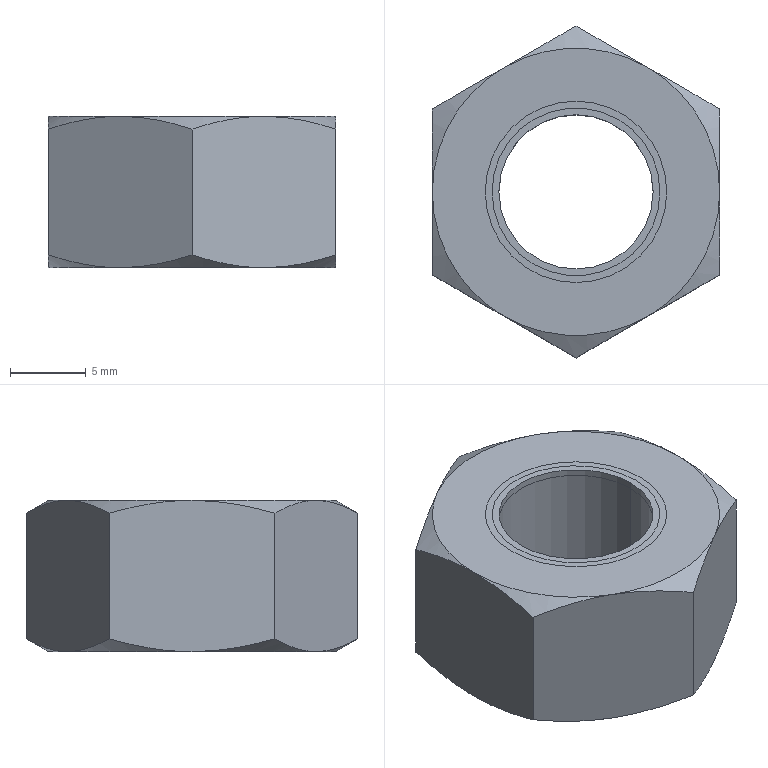Part | STEP file | M12 | 2 solids | 32 faces | box 19 x 21.939 x 10 mm | volume 2601 mm3 | cone 16 | plane 10 | cylinder 6 | commonest cylinder face diameters 10.2 x4 12 x2
STEP:
#1=CARTESIAN_POINT('',(5.1,0.,9.55));
#2=VERTEX_POINT('',#1);
#3=CARTESIAN_POINT('',(-5.1,0.,9.55));
#4=VERTEX_POINT('',#3);
#5=CARTESIAN_POINT('',(0.,0.,9.55));
#6=DIRECTION('',(0.,0.,-1.));
#7=DIRECTION('',(1.,0.,0.));
#8=AXIS2_PLACEMENT_3D('',#5,#6,#7);
#9=CIRCLE('',#8,5.1);
#10=EDGE_CURVE('',#2,#4,#9,.T.);
#11=ORIENTED_EDGE('',*,*,#10,.F.);
#12=CARTESIAN_POINT('',(5.1,0.,0.45));
#13=VERTEX_POINT('',#12);
#14=CARTESIAN_POINT('',(5.1,0.,0.));
#15=DIRECTION('',(0.,0.,-1.));
#16=VECTOR('',#15,1000.);
#17=LINE('',#14,#16);
#18=EDGE_CURVE('',#2,#13,#17,.T.);
#19=ORIENTED_EDGE('',*,*,#18,.T.);
#20=CARTESIAN_POINT('',(-5.1,0.,0.45));
#21=VERTEX_POINT('',#20);
#22=CARTESIAN_POINT('',(0.,0.,0.45));
#23=DIRECTION('',(0.,0.,1.));
#24=DIRECTION('',(-1.,0.,0.));
#25=AXIS2_PLACEMENT_3D('',#22,#23,#24);
#26=CIRCLE('',#25,5.1);
#27=EDGE_CURVE('',#21,#13,#26,.T.);
#28=ORIENTED_EDGE('',*,*,#27,.F.);
#29=CARTESIAN_POINT('',(-5.1,0.,0.));
#30=DIRECTION('',(0.,0.,-1.));
#31=VECTOR('',#30,1000.);
#32=LINE('',#29,#31);
#33=EDGE_CURVE('',#4,#21,#32,.T.);
#34=ORIENTED_EDGE('',*,*,#33,.F.);
#35=EDGE_LOOP('',(#11,#19,#28,#34));
#36=FACE_OUTER_BOUND('',#35,.T.);
#37=CARTESIAN_POINT('',(0.,0.,0.));
#38=DIRECTION('',(0.,0.,-1.));
#39=DIRECTION('',(-1.,0.,0.));
#40=AXIS2_PLACEMENT_3D('',#37,#38,#39);
#41=CYLINDRICAL_SURFACE('',#40,5.1);
#42=ADVANCED_FACE('',(#36),#41,.F.);
#43=ORIENTED_EDGE('',*,*,#27,.T.);
#44=CARTESIAN_POINT('',(5.55,0.,0.));
#45=VERTEX_POINT('',#44);
#46=CARTESIAN_POINT('',(5.55,0.,0.000002816));
#47=DIRECTION('',(0.7071,0.,-0.7071));
#48=VECTOR('',#47,1000.);
#49=LINE('',#46,#48);
#50=EDGE_CURVE('',#13,#45,#49,.T.);
#51=ORIENTED_EDGE('',*,*,#50,.T.);
#52=CARTESIAN_POINT('',(-5.55,0.,0.));
#53=VERTEX_POINT('',#52);
#54=CARTESIAN_POINT('',(0.,0.,0.));
#55=DIRECTION('',(0.,0.,-1.));
#56=DIRECTION('',(1.,0.,0.));
#57=AXIS2_PLACEMENT_3D('',#54,#55,#56);
#58=CIRCLE('',#57,5.55);
#59=EDGE_CURVE('',#45,#53,#58,.T.);
#60=ORIENTED_EDGE('',*,*,#59,.T.);
#61=CARTESIAN_POINT('',(-5.55,0.,0.000002816));
#62=DIRECTION('',(-0.7071,0.,-0.7071));
#63=VECTOR('',#62,1000.);
#64=LINE('',#61,#63);
#65=EDGE_CURVE('',#21,#53,#64,.T.);
#66=ORIENTED_EDGE('',*,*,#65,.F.);
#67=EDGE_LOOP('',(#43,#51,#60,#66));
#68=FACE_OUTER_BOUND('',#67,.T.);
#69=CARTESIAN_POINT('',(0.,0.,0.000002816));
#70=DIRECTION('',(0.,0.,-1.));
#71=DIRECTION('',(-1.,0.,0.));
#72=AXIS2_PLACEMENT_3D('',#69,#70,#71);
#73=CONICAL_SURFACE('',#72,5.55,0.7854);
#74=ADVANCED_FACE('',(#68),#73,.F.);
#75=ORIENTED_EDGE('',*,*,#10,.T.);
#76=CARTESIAN_POINT('',(-5.55,0.,10.));
#77=VERTEX_POINT('',#76);
#78=CARTESIAN_POINT('',(-5.55,0.,10.));
#79=DIRECTION('',(-0.7071,0.,0.7071));
#80=VECTOR('',#79,1000.);
#81=LINE('',#78,#80);
#82=EDGE_CURVE('',#4,#77,#81,.T.);
#83=ORIENTED_EDGE('',*,*,#82,.T.);
#84=CARTESIAN_POINT('',(5.55,0.,10.));
#85=VERTEX_POINT('',#84);
#86=CARTESIAN_POINT('',(0.,0.,10.));
#87=DIRECTION('',(0.,0.,-1.));
#88=DIRECTION('',(1.,0.,0.));
#89=AXIS2_PLACEMENT_3D('',#86,#87,#88);
#90=CIRCLE('',#89,5.55);
#91=EDGE_CURVE('',#85,#77,#90,.T.);
#92=ORIENTED_EDGE('',*,*,#91,.F.);
#93=CARTESIAN_POINT('',(5.55,0.,10.));
#94=DIRECTION('',(0.7071,0.,0.7071));
#95=VECTOR('',#94,1000.);
#96=LINE('',#93,#95);
#97=EDGE_CURVE('',#2,#85,#96,.T.);
#98=ORIENTED_EDGE('',*,*,#97,.F.);
#99=EDGE_LOOP('',(#75,#83,#92,#98));
#100=FACE_OUTER_BOUND('',#99,.T.);
#101=CARTESIAN_POINT('',(0.,0.,10.));
#102=DIRECTION('',(0.,0.,1.));
#103=DIRECTION('',(1.,0.,0.));
#104=AXIS2_PLACEMENT_3D('',#101,#102,#103);
#105=CONICAL_SURFACE('',#104,5.55,0.7854);
#106=ADVANCED_FACE('',(#100),#105,.F.);
#107=CARTESIAN_POINT('',(0.,0.,0.));
#108=DIRECTION('',(0.,0.,-1.));
#109=DIRECTION('',(1.,0.,0.));
#110=AXIS2_PLACEMENT_3D('',#107,#108,#109);
#111=CIRCLE('',#110,5.55);
#112=EDGE_CURVE('',#53,#45,#111,.T.);
#113=ORIENTED_EDGE('',*,*,#112,.F.);
#114=ORIENTED_EDGE('',*,*,#59,.F.);
#115=EDGE_LOOP('',(#113,#114));
#116=FACE_BOUND('',#115,.T.);
#117=CARTESIAN_POINT('',(-4.75,8.227,0.));
#118=VERTEX_POINT('',#117);
#119=CARTESIAN_POINT('',(-9.5,0.,0.));
#120=VERTEX_POINT('',#119);
#121=CARTESIAN_POINT('',(0.,0.,0.));
#122=DIRECTION('',(0.,0.,1.));
#123=DIRECTION('',(1.,0.,0.));
#124=AXIS2_PLACEMENT_3D('',#121,#122,#123);
#125=CIRCLE('',#124,9.5);
#126=EDGE_CURVE('',#118,#120,#125,.T.);
#127=ORIENTED_EDGE('',*,*,#126,.F.);
#128=CARTESIAN_POINT('',(4.75,8.227,0.));
#129=VERTEX_POINT('',#128);
#130=CARTESIAN_POINT('',(0.,0.,0.));
#131=DIRECTION('',(0.,0.,1.));
#132=DIRECTION('',(1.,0.,0.));
#133=AXIS2_PLACEMENT_3D('',#130,#131,#132);
#134=CIRCLE('',#133,9.5);
#135=EDGE_CURVE('',#129,#118,#134,.T.);
#136=ORIENTED_EDGE('',*,*,#135,.F.);
#137=CARTESIAN_POINT('',(9.5,0.000000041,0.));
#138=VERTEX_POINT('',#137);
#139=CARTESIAN_POINT('',(0.,0.,0.000000001));
#140=DIRECTION('',(0.,0.,1.));
#141=DIRECTION('',(1.,0.,0.));
#142=AXIS2_PLACEMENT_3D('',#139,#140,#141);
#143=CIRCLE('',#142,9.5);
#144=EDGE_CURVE('',#138,#129,#143,.T.);
#145=ORIENTED_EDGE('',*,*,#144,.F.);
#146=CARTESIAN_POINT('',(4.75,-8.227,0.));
#147=VERTEX_POINT('',#146);
#148=CARTESIAN_POINT('',(0.,0.,0.));
#149=DIRECTION('',(0.,0.,1.));
#150=DIRECTION('',(1.,0.,0.));
#151=AXIS2_PLACEMENT_3D('',#148,#149,#150);
#152=CIRCLE('',#151,9.5);
#153=EDGE_CURVE('',#147,#138,#152,.T.);
#154=ORIENTED_EDGE('',*,*,#153,.F.);
#155=CARTESIAN_POINT('',(-4.75,-8.227,0.));
#156=VERTEX_POINT('',#155);
#157=CARTESIAN_POINT('',(0.,0.,0.));
#158=DIRECTION('',(0.,0.,1.));
#159=DIRECTION('',(1.,0.,0.));
#160=AXIS2_PLACEMENT_3D('',#157,#158,#159);
#161=CIRCLE('',#160,9.5);
#162=EDGE_CURVE('',#156,#147,#161,.T.);
#163=ORIENTED_EDGE('',*,*,#162,.F.);
#164=CARTESIAN_POINT('',(0.,0.,0.));
#165=DIRECTION('',(0.,0.,1.));
#166=DIRECTION('',(1.,0.,0.));
#167=AXIS2_PLACEMENT_3D('',#164,#165,#166);
#168=CIRCLE('',#167,9.5);
#169=EDGE_CURVE('',#120,#156,#168,.T.);
#170=ORIENTED_EDGE('',*,*,#169,.F.);
#171=EDGE_LOOP('',(#127,#136,#145,#154,#163,#170));
#172=FACE_OUTER_BOUND('',#171,.T.);
#173=CARTESIAN_POINT('',(0.,0.,0.));
#174=DIRECTION('',(0.,0.,1.));
#175=DIRECTION('',(1.,0.,0.));
#176=AXIS2_PLACEMENT_3D('',#173,#174,#175);
#177=PLANE('',#176);
#178=ADVANCED_FACE('',(#116,#172),#177,.F.);
#179=ORIENTED_EDGE('',*,*,#50,.F.);
#180=CARTESIAN_POINT('',(0.,0.,0.45));
#181=DIRECTION('',(0.,0.,1.));
#182=DIRECTION('',(-1.,0.,0.));
#183=AXIS2_PLACEMENT_3D('',#180,#181,#182);
#184=CIRCLE('',#183,5.1);
#185=EDGE_CURVE('',#13,#21,#184,.T.);
#186=ORIENTED_EDGE('',*,*,#185,.T.);
#187=ORIENTED_EDGE('',*,*,#65,.T.);
#188=ORIENTED_EDGE('',*,*,#112,.T.);
#189=EDGE_LOOP('',(#179,#186,#187,#188));
#190=FACE_OUTER_BOUND('',#189,.T.);
#191=CARTESIAN_POINT('',(0.,0.,0.000002816));
#192=DIRECTION('',(0.,0.,-1.));
#193=DIRECTION('',(-1.,0.,0.));
#194=AXIS2_PLACEMENT_3D('',#191,#192,#193);
#195=CONICAL_SURFACE('',#194,5.55,0.7854);
#196=ADVANCED_FACE('',(#190),#195,.F.);
#197=CARTESIAN_POINT('',(-9.5,-5.485,0.8485));
#198=VERTEX_POINT('',#197);
#199=CARTESIAN_POINT('',(-4.75,-8.227,0.));
#200=CARTESIAN_POINT('',(-5.561,-7.759,0.));
#201=CARTESIAN_POINT('',(-6.36,-7.298,0.08112));
#202=CARTESIAN_POINT('',(-7.942,-6.384,0.3765));
#203=CARTESIAN_POINT('',(-8.724,-5.933,0.5899));
#204=CARTESIAN_POINT('',(-9.5,-5.485,0.8485));
#205=B_SPLINE_CURVE_WITH_KNOTS('',3,(#199,#200,#201,#202,#203,#204),.UNSPECIFIED.,.F.,.F.,(4,2,4),(0.,0.002775,0.00555),.UNSPECIFIED.);
#206=EDGE_CURVE('',#156,#198,#205,.T.);
#207=ORIENTED_EDGE('',*,*,#206,.T.);
#208=CARTESIAN_POINT('',(-9.5,-5.485,0.8485));
#209=CARTESIAN_POINT('',(-9.5,-4.589,0.5899));
#210=CARTESIAN_POINT('',(-9.5,-3.686,0.3765));
#211=CARTESIAN_POINT('',(-9.5,-1.859,0.08112));
#212=CARTESIAN_POINT('',(-9.5,-0.936,0.));
#213=CARTESIAN_POINT('',(-9.5,0.,0.));
#214=B_SPLINE_CURVE_WITH_KNOTS('',3,(#208,#209,#210,#211,#212,#213),.UNSPECIFIED.,.F.,.F.,(4,2,4),(0.,0.002775,0.00555),.UNSPECIFIED.);
#215=EDGE_CURVE('',#198,#120,#214,.T.);
#216=ORIENTED_EDGE('',*,*,#215,.T.);
#217=ORIENTED_EDGE('',*,*,#169,.T.);
#218=EDGE_LOOP('',(#207,#216,#217));
#219=FACE_OUTER_BOUND('',#218,.T.);
#220=CARTESIAN_POINT('',(0.,0.,0.8536));
#221=DIRECTION('',(0.,0.,1.));
#222=DIRECTION('',(1.,0.,0.));
#223=AXIS2_PLACEMENT_3D('',#220,#221,#222);
#224=CONICAL_SURFACE('',#223,10.978,1.047);
#225=ADVANCED_FACE('',(#219),#224,.T.);
#226=CARTESIAN_POINT('',(-9.5,5.485,0.8485));
#227=VERTEX_POINT('',#226);
#228=CARTESIAN_POINT('',(-9.5,0.,0.));
#229=CARTESIAN_POINT('',(-9.5,0.936,0.));
#230=CARTESIAN_POINT('',(-9.5,1.859,0.08112));
#231=CARTESIAN_POINT('',(-9.5,3.686,0.3765));
#232=CARTESIAN_POINT('',(-9.5,4.589,0.5899));
#233=CARTESIAN_POINT('',(-9.5,5.485,0.8485));
#234=B_SPLINE_CURVE_WITH_KNOTS('',3,(#228,#229,#230,#231,#232,#233),.UNSPECIFIED.,.F.,.F.,(4,2,4),(0.,0.002775,0.00555),.UNSPECIFIED.);
#235=EDGE_CURVE('',#120,#227,#234,.T.);
#236=ORIENTED_EDGE('',*,*,#235,.T.);
#237=CARTESIAN_POINT('',(-9.5,5.485,0.8485));
#238=CARTESIAN_POINT('',(-8.724,5.933,0.5899));
#239=CARTESIAN_POINT('',(-7.942,6.384,0.3765));
#240=CARTESIAN_POINT('',(-6.36,7.298,0.08112));
#241=CARTESIAN_POINT('',(-5.561,7.759,0.));
#242=CARTESIAN_POINT('',(-4.75,8.227,0.));
#243=B_SPLINE_CURVE_WITH_KNOTS('',3,(#237,#238,#239,#240,#241,#242),.UNSPECIFIED.,.F.,.F.,(4,2,4),(0.,0.002775,0.00555),.UNSPECIFIED.);
#244=EDGE_CURVE('',#227,#118,#243,.T.);
#245=ORIENTED_EDGE('',*,*,#244,.T.);
#246=ORIENTED_EDGE('',*,*,#126,.T.);
#247=EDGE_LOOP('',(#236,#245,#246));
#248=FACE_OUTER_BOUND('',#247,.T.);
#249=CARTESIAN_POINT('',(0.,0.,0.8536));
#250=DIRECTION('',(0.,0.,1.));
#251=DIRECTION('',(1.,0.,0.));
#252=AXIS2_PLACEMENT_3D('',#249,#250,#251);
#253=CONICAL_SURFACE('',#252,10.978,1.047);
#254=ADVANCED_FACE('',(#248),#253,.T.);
#255=CARTESIAN_POINT('',(-0.000000038,10.97,0.8485));
#256=VERTEX_POINT('',#255);
#257=CARTESIAN_POINT('',(-4.75,8.227,0.));
#258=CARTESIAN_POINT('',(-3.939,8.695,0.));
#259=CARTESIAN_POINT('',(-3.14,9.157,0.08112));
#260=CARTESIAN_POINT('',(-1.558,10.07,0.3765));
#261=CARTESIAN_POINT('',(-0.776,10.522,0.5899));
#262=CARTESIAN_POINT('',(-0.000000038,10.97,0.8485));
#263=B_SPLINE_CURVE_WITH_KNOTS('',3,(#257,#258,#259,#260,#261,#262),.UNSPECIFIED.,.F.,.F.,(4,2,4),(0.,0.002775,0.00555),.UNSPECIFIED.);
#264=EDGE_CURVE('',#118,#256,#263,.T.);
#265=ORIENTED_EDGE('',*,*,#264,.T.);
#266=CARTESIAN_POINT('',(-0.000000038,10.97,0.8485));
#267=CARTESIAN_POINT('',(0.776,10.522,0.5899));
#268=CARTESIAN_POINT('',(1.558,10.07,0.3765));
#269=CARTESIAN_POINT('',(3.14,9.157,0.08112));
#270=CARTESIAN_POINT('',(3.939,8.695,0.));
#271=CARTESIAN_POINT('',(4.75,8.227,0.));
#272=B_SPLINE_CURVE_WITH_KNOTS('',3,(#266,#267,#268,#269,#270,#271),.UNSPECIFIED.,.F.,.F.,(4,2,4),(0.,0.002775,0.00555),.UNSPECIFIED.);
#273=EDGE_CURVE('',#256,#129,#272,.T.);
#274=ORIENTED_EDGE('',*,*,#273,.T.);
#275=ORIENTED_EDGE('',*,*,#135,.T.);
#276=EDGE_LOOP('',(#265,#274,#275));
#277=FACE_OUTER_BOUND('',#276,.T.);
#278=CARTESIAN_POINT('',(0.,0.,0.8536));
#279=DIRECTION('',(0.,0.,1.));
#280=DIRECTION('',(1.,0.,0.));
#281=AXIS2_PLACEMENT_3D('',#278,#279,#280);
#282=CONICAL_SURFACE('',#281,10.978,1.047);
#283=ADVANCED_FACE('',(#277),#282,.T.);
#284=CARTESIAN_POINT('',(9.5,5.485,0.8485));
#285=VERTEX_POINT('',#284);
#286=CARTESIAN_POINT('',(4.75,8.227,0.));
#287=CARTESIAN_POINT('',(5.561,7.759,0.));
#288=CARTESIAN_POINT('',(6.36,7.298,0.08112));
#289=CARTESIAN_POINT('',(7.942,6.384,0.3765));
#290=CARTESIAN_POINT('',(8.724,5.933,0.5899));
#291=CARTESIAN_POINT('',(9.5,5.485,0.8485));
#292=B_SPLINE_CURVE_WITH_KNOTS('',3,(#286,#287,#288,#289,#290,#291),.UNSPECIFIED.,.F.,.F.,(4,2,4),(0.,0.002775,0.00555),.UNSPECIFIED.);
#293=EDGE_CURVE('',#129,#285,#292,.T.);
#294=ORIENTED_EDGE('',*,*,#293,.T.);
#295=CARTESIAN_POINT('',(9.5,5.485,0.8485));
#296=CARTESIAN_POINT('',(9.5,4.589,0.5899));
#297=CARTESIAN_POINT('',(9.5,3.686,0.3765));
#298=CARTESIAN_POINT('',(9.5,1.859,0.08112));
#299=CARTESIAN_POINT('',(9.5,0.936,0.000000002));
#300=CARTESIAN_POINT('',(9.5,0.000000041,0.));
#301=B_SPLINE_CURVE_WITH_KNOTS('',3,(#295,#296,#297,#298,#299,#300),.UNSPECIFIED.,.F.,.F.,(4,2,4),(0.,0.002775,0.00555),.UNSPECIFIED.);
#302=EDGE_CURVE('',#285,#138,#301,.T.);
#303=ORIENTED_EDGE('',*,*,#302,.T.);
#304=ORIENTED_EDGE('',*,*,#144,.T.);
#305=EDGE_LOOP('',(#294,#303,#304));
#306=FACE_OUTER_BOUND('',#305,.T.);
#307=CARTESIAN_POINT('',(0.,0.,0.8536));
#308=DIRECTION('',(0.,0.,1.));
#309=DIRECTION('',(1.,0.,0.));
#310=AXIS2_PLACEMENT_3D('',#307,#308,#309);
#311=CONICAL_SURFACE('',#310,10.978,1.047);
#312=ADVANCED_FACE('',(#306),#311,.T.);
#313=CARTESIAN_POINT('',(9.5,-5.485,0.8485));
#314=VERTEX_POINT('',#313);
#315=CARTESIAN_POINT('',(9.5,0.000000041,0.));
#316=CARTESIAN_POINT('',(9.5,-0.936,-0.000000002));
#317=CARTESIAN_POINT('',(9.5,-1.859,0.08112));
#318=CARTESIAN_POINT('',(9.5,-3.686,0.3765));
#319=CARTESIAN_POINT('',(9.5,-4.589,0.5899));
#320=CARTESIAN_POINT('',(9.5,-5.485,0.8485));
#321=B_SPLINE_CURVE_WITH_KNOTS('',3,(#315,#316,#317,#318,#319,#320),.UNSPECIFIED.,.F.,.F.,(4,2,4),(0.,0.002775,0.00555),.UNSPECIFIED.);
#322=EDGE_CURVE('',#138,#314,#321,.T.);
#323=ORIENTED_EDGE('',*,*,#322,.T.);
#324=CARTESIAN_POINT('',(9.5,-5.485,0.8485));
#325=CARTESIAN_POINT('',(8.724,-5.933,0.5899));
#326=CARTESIAN_POINT('',(7.942,-6.384,0.3765));
#327=CARTESIAN_POINT('',(6.36,-7.298,0.08112));
#328=CARTESIAN_POINT('',(5.561,-7.759,0.));
#329=CARTESIAN_POINT('',(4.75,-8.227,0.));
#330=B_SPLINE_CURVE_WITH_KNOTS('',3,(#324,#325,#326,#327,#328,#329),.UNSPECIFIED.,.F.,.F.,(4,2,4),(0.,0.002775,0.00555),.UNSPECIFIED.);
#331=EDGE_CURVE('',#314,#147,#330,.T.);
#332=ORIENTED_EDGE('',*,*,#331,.T.);
#333=ORIENTED_EDGE('',*,*,#153,.T.);
#334=EDGE_LOOP('',(#323,#332,#333));
#335=FACE_OUTER_BOUND('',#334,.T.);
#336=CARTESIAN_POINT('',(0.,0.,0.8536));
#337=DIRECTION('',(0.,0.,1.));
#338=DIRECTION('',(1.,0.,0.));
#339=AXIS2_PLACEMENT_3D('',#336,#337,#338);
#340=CONICAL_SURFACE('',#339,10.978,1.047);
#341=ADVANCED_FACE('',(#335),#340,.T.);
#342=CARTESIAN_POINT('',(0.000000038,-10.97,0.8485));
#343=VERTEX_POINT('',#342);
#344=CARTESIAN_POINT('',(4.75,-8.227,0.));
#345=CARTESIAN_POINT('',(3.939,-8.695,0.));
#346=CARTESIAN_POINT('',(3.14,-9.157,0.08112));
#347=CARTESIAN_POINT('',(1.558,-10.07,0.3765));
#348=CARTESIAN_POINT('',(0.776,-10.522,0.5899));
#349=CARTESIAN_POINT('',(0.000000038,-10.97,0.8485));
#350=B_SPLINE_CURVE_WITH_KNOTS('',3,(#344,#345,#346,#347,#348,#349),.UNSPECIFIED.,.F.,.F.,(4,2,4),(0.,0.002775,0.00555),.UNSPECIFIED.);
#351=EDGE_CURVE('',#147,#343,#350,.T.);
#352=ORIENTED_EDGE('',*,*,#351,.T.);
#353=CARTESIAN_POINT('',(0.000000038,-10.97,0.8485));
#354=CARTESIAN_POINT('',(-0.776,-10.522,0.5899));
#355=CARTESIAN_POINT('',(-1.558,-10.07,0.3765));
#356=CARTESIAN_POINT('',(-3.14,-9.157,0.08112));
#357=CARTESIAN_POINT('',(-3.939,-8.695,0.));
#358=CARTESIAN_POINT('',(-4.75,-8.227,0.));
#359=B_SPLINE_CURVE_WITH_KNOTS('',3,(#353,#354,#355,#356,#357,#358),.UNSPECIFIED.,.F.,.F.,(4,2,4),(0.,0.002775,0.00555),.UNSPECIFIED.);
#360=EDGE_CURVE('',#343,#156,#359,.T.);
#361=ORIENTED_EDGE('',*,*,#360,.T.);
#362=ORIENTED_EDGE('',*,*,#162,.T.);
#363=EDGE_LOOP('',(#352,#361,#362));
#364=FACE_OUTER_BOUND('',#363,.T.);
#365=CARTESIAN_POINT('',(0.,0.,0.8536));
#366=DIRECTION('',(0.,0.,1.));
#367=DIRECTION('',(1.,0.,0.));
#368=AXIS2_PLACEMENT_3D('',#365,#366,#367);
#369=CONICAL_SURFACE('',#368,10.978,1.047);
#370=ADVANCED_FACE('',(#364),#369,.T.);
#371=ORIENTED_EDGE('',*,*,#235,.F.);
#372=ORIENTED_EDGE('',*,*,#215,.F.);
#373=CARTESIAN_POINT('',(-9.5,-5.485,9.151));
#374=VERTEX_POINT('',#373);
#375=CARTESIAN_POINT('',(-9.5,-5.485,0.));
#376=DIRECTION('',(0.,0.,1.));
#377=VECTOR('',#376,1000.);
#378=LINE('',#375,#377);
#379=EDGE_CURVE('',#198,#374,#378,.T.);
#380=ORIENTED_EDGE('',*,*,#379,.T.);
#381=CARTESIAN_POINT('',(-9.5,0.,10.));
#382=VERTEX_POINT('',#381);
#383=CARTESIAN_POINT('',(-9.5,-5.485,9.151));
#384=CARTESIAN_POINT('',(-9.5,-4.589,9.41));
#385=CARTESIAN_POINT('',(-9.5,-3.686,9.623));
#386=CARTESIAN_POINT('',(-9.5,-1.859,9.919));
#387=CARTESIAN_POINT('',(-9.5,-0.936,10.));
#388=CARTESIAN_POINT('',(-9.5,0.,10.));
#389=B_SPLINE_CURVE_WITH_KNOTS('',3,(#383,#384,#385,#386,#387,#388),.UNSPECIFIED.,.F.,.F.,(4,2,4),(0.,0.002775,0.00555),.UNSPECIFIED.);
#390=EDGE_CURVE('',#374,#382,#389,.T.);
#391=ORIENTED_EDGE('',*,*,#390,.T.);
#392=CARTESIAN_POINT('',(-9.5,5.485,9.151));
#393=VERTEX_POINT('',#392);
#394=CARTESIAN_POINT('',(-9.5,0.,10.));
#395=CARTESIAN_POINT('',(-9.5,0.936,10.));
#396=CARTESIAN_POINT('',(-9.5,1.859,9.919));
#397=CARTESIAN_POINT('',(-9.5,3.686,9.623));
#398=CARTESIAN_POINT('',(-9.5,4.589,9.41));
#399=CARTESIAN_POINT('',(-9.5,5.485,9.151));
#400=B_SPLINE_CURVE_WITH_KNOTS('',3,(#394,#395,#396,#397,#398,#399),.UNSPECIFIED.,.F.,.F.,(4,2,4),(0.,0.002775,0.00555),.UNSPECIFIED.);
#401=EDGE_CURVE('',#382,#393,#400,.T.);
#402=ORIENTED_EDGE('',*,*,#401,.T.);
#403=CARTESIAN_POINT('',(-9.5,5.485,0.));
#404=DIRECTION('',(0.,0.,-1.));
#405=VECTOR('',#404,1000.);
#406=LINE('',#403,#405);
#407=EDGE_CURVE('',#393,#227,#406,.T.);
#408=ORIENTED_EDGE('',*,*,#407,.T.);
#409=EDGE_LOOP('',(#371,#372,#380,#391,#402,#408));
#410=FACE_OUTER_BOUND('',#409,.T.);
#411=CARTESIAN_POINT('',(-9.5,5.485,0.));
#412=DIRECTION('',(-1.,0.,0.));
#413=DIRECTION('',(0.,0.,1.));
#414=AXIS2_PLACEMENT_3D('',#411,#412,#413);
#415=PLANE('',#414);
#416=ADVANCED_FACE('',(#410),#415,.T.);
#417=ORIENTED_EDGE('',*,*,#206,.F.);
#418=ORIENTED_EDGE('',*,*,#360,.F.);
#419=CARTESIAN_POINT('',(0.,-10.97,9.151));
#420=VERTEX_POINT('',#419);
#421=CARTESIAN_POINT('',(0.,-10.97,0.));
#422=DIRECTION('',(0.,0.,1.));
#423=VECTOR('',#422,1000.);
#424=LINE('',#421,#423);
#425=EDGE_CURVE('',#343,#420,#424,.T.);
#426=ORIENTED_EDGE('',*,*,#425,.T.);
#427=CARTESIAN_POINT('',(-4.75,-8.227,10.));
#428=VERTEX_POINT('',#427);
#429=CARTESIAN_POINT('',(0.,-10.97,9.151));
#430=CARTESIAN_POINT('',(-0.776,-10.522,9.41));
#431=CARTESIAN_POINT('',(-1.558,-10.07,9.623));
#432=CARTESIAN_POINT('',(-3.14,-9.157,9.919));
#433=CARTESIAN_POINT('',(-3.939,-8.695,10.));
#434=CARTESIAN_POINT('',(-4.75,-8.227,10.));
#435=B_SPLINE_CURVE_WITH_KNOTS('',3,(#429,#430,#431,#432,#433,#434),.UNSPECIFIED.,.F.,.F.,(4,2,4),(0.,0.002775,0.00555),.UNSPECIFIED.);
#436=EDGE_CURVE('',#420,#428,#435,.T.);
#437=ORIENTED_EDGE('',*,*,#436,.T.);
#438=CARTESIAN_POINT('',(-4.75,-8.227,10.));
#439=CARTESIAN_POINT('',(-5.561,-7.759,10.));
#440=CARTESIAN_POINT('',(-6.36,-7.298,9.919));
#441=CARTESIAN_POINT('',(-7.942,-6.384,9.623));
#442=CARTESIAN_POINT('',(-8.724,-5.933,9.41));
#443=CARTESIAN_POINT('',(-9.5,-5.485,9.151));
#444=B_SPLINE_CURVE_WITH_KNOTS('',3,(#438,#439,#440,#441,#442,#443),.UNSPECIFIED.,.F.,.F.,(4,2,4),(0.,0.002775,0.00555),.UNSPECIFIED.);
#445=EDGE_CURVE('',#428,#374,#444,.T.);
#446=ORIENTED_EDGE('',*,*,#445,.T.);
#447=ORIENTED_EDGE('',*,*,#379,.F.);
#448=EDGE_LOOP('',(#417,#418,#426,#437,#446,#447));
#449=FACE_OUTER_BOUND('',#448,.T.);
#450=CARTESIAN_POINT('',(-9.5,-5.485,0.));
#451=DIRECTION('',(-0.5,-0.866,0.));
#452=DIRECTION('',(0.866,-0.5,0.));
#453=AXIS2_PLACEMENT_3D('',#450,#451,#452);
#454=PLANE('',#453);
#455=ADVANCED_FACE('',(#449),#454,.T.);
#456=ORIENTED_EDGE('',*,*,#264,.F.);
#457=ORIENTED_EDGE('',*,*,#244,.F.);
#458=ORIENTED_EDGE('',*,*,#407,.F.);
#459=CARTESIAN_POINT('',(-4.75,8.227,10.));
#460=VERTEX_POINT('',#459);
#461=CARTESIAN_POINT('',(-9.5,5.485,9.151));
#462=CARTESIAN_POINT('',(-8.724,5.933,9.41));
#463=CARTESIAN_POINT('',(-7.942,6.384,9.623));
#464=CARTESIAN_POINT('',(-6.36,7.298,9.919));
#465=CARTESIAN_POINT('',(-5.561,7.759,10.));
#466=CARTESIAN_POINT('',(-4.75,8.227,10.));
#467=B_SPLINE_CURVE_WITH_KNOTS('',3,(#461,#462,#463,#464,#465,#466),.UNSPECIFIED.,.F.,.F.,(4,2,4),(0.,0.002775,0.00555),.UNSPECIFIED.);
#468=EDGE_CURVE('',#393,#460,#467,.T.);
#469=ORIENTED_EDGE('',*,*,#468,.T.);
#470=CARTESIAN_POINT('',(0.,10.97,9.151));
#471=VERTEX_POINT('',#470);
#472=CARTESIAN_POINT('',(-4.75,8.227,10.));
#473=CARTESIAN_POINT('',(-3.939,8.695,10.));
#474=CARTESIAN_POINT('',(-3.14,9.157,9.919));
#475=CARTESIAN_POINT('',(-1.558,10.07,9.623));
#476=CARTESIAN_POINT('',(-0.776,10.522,9.41));
#477=CARTESIAN_POINT('',(0.,10.97,9.151));
#478=B_SPLINE_CURVE_WITH_KNOTS('',3,(#472,#473,#474,#475,#476,#477),.UNSPECIFIED.,.F.,.F.,(4,2,4),(0.,0.002775,0.00555),.UNSPECIFIED.);
#479=EDGE_CURVE('',#460,#471,#478,.T.);
#480=ORIENTED_EDGE('',*,*,#479,.T.);
#481=CARTESIAN_POINT('',(0.,10.97,0.));
#482=DIRECTION('',(0.,0.,-1.));
#483=VECTOR('',#482,1000.);
#484=LINE('',#481,#483);
#485=EDGE_CURVE('',#471,#256,#484,.T.);
#486=ORIENTED_EDGE('',*,*,#485,.T.);
#487=EDGE_LOOP('',(#456,#457,#458,#469,#480,#486));
#488=FACE_OUTER_BOUND('',#487,.T.);
#489=CARTESIAN_POINT('',(0.,10.97,0.));
#490=DIRECTION('',(-0.5,0.866,0.));
#491=DIRECTION('',(-0.866,-0.5,0.));
#492=AXIS2_PLACEMENT_3D('',#489,#490,#491);
#493=PLANE('',#492);
#494=ADVANCED_FACE('',(#488),#493,.T.);
#495=ORIENTED_EDGE('',*,*,#293,.F.);
#496=ORIENTED_EDGE('',*,*,#273,.F.);
#497=ORIENTED_EDGE('',*,*,#485,.F.);
#498=CARTESIAN_POINT('',(4.75,8.227,10.));
#499=VERTEX_POINT('',#498);
#500=CARTESIAN_POINT('',(0.,10.97,9.151));
#501=CARTESIAN_POINT('',(0.776,10.522,9.41));
#502=CARTESIAN_POINT('',(1.558,10.07,9.623));
#503=CARTESIAN_POINT('',(3.14,9.157,9.919));
#504=CARTESIAN_POINT('',(3.939,8.695,10.));
#505=CARTESIAN_POINT('',(4.75,8.227,10.));
#506=B_SPLINE_CURVE_WITH_KNOTS('',3,(#500,#501,#502,#503,#504,#505),.UNSPECIFIED.,.F.,.F.,(4,2,4),(0.,0.002775,0.00555),.UNSPECIFIED.);
#507=EDGE_CURVE('',#471,#499,#506,.T.);
#508=ORIENTED_EDGE('',*,*,#507,.T.);
#509=CARTESIAN_POINT('',(9.5,5.485,9.151));
#510=VERTEX_POINT('',#509);
#511=CARTESIAN_POINT('',(4.75,8.227,10.));
#512=CARTESIAN_POINT('',(5.561,7.759,10.));
#513=CARTESIAN_POINT('',(6.36,7.298,9.919));
#514=CARTESIAN_POINT('',(7.942,6.384,9.623));
#515=CARTESIAN_POINT('',(8.724,5.933,9.41));
#516=CARTESIAN_POINT('',(9.5,5.485,9.151));
#517=B_SPLINE_CURVE_WITH_KNOTS('',3,(#511,#512,#513,#514,#515,#516),.UNSPECIFIED.,.F.,.F.,(4,2,4),(0.,0.002775,0.00555),.UNSPECIFIED.);
#518=EDGE_CURVE('',#499,#510,#517,.T.);
#519=ORIENTED_EDGE('',*,*,#518,.T.);
#520=CARTESIAN_POINT('',(9.5,5.485,0.));
#521=DIRECTION('',(0.,0.,-1.));
#522=VECTOR('',#521,1000.);
#523=LINE('',#520,#522);
#524=EDGE_CURVE('',#510,#285,#523,.T.);
#525=ORIENTED_EDGE('',*,*,#524,.T.);
#526=EDGE_LOOP('',(#495,#496,#497,#508,#519,#525));
#527=FACE_OUTER_BOUND('',#526,.T.);
#528=CARTESIAN_POINT('',(9.5,5.485,0.));
#529=DIRECTION('',(0.5,0.866,0.));
#530=DIRECTION('',(-0.866,0.5,0.));
#531=AXIS2_PLACEMENT_3D('',#528,#529,#530);
#532=PLANE('',#531);
#533=ADVANCED_FACE('',(#527),#532,.T.);
#534=ORIENTED_EDGE('',*,*,#322,.F.);
#535=ORIENTED_EDGE('',*,*,#302,.F.);
#536=ORIENTED_EDGE('',*,*,#524,.F.);
#537=CARTESIAN_POINT('',(9.5,0.,10.));
#538=VERTEX_POINT('',#537);
#539=CARTESIAN_POINT('',(9.5,5.485,9.151));
#540=CARTESIAN_POINT('',(9.5,4.589,9.41));
#541=CARTESIAN_POINT('',(9.5,3.686,9.623));
#542=CARTESIAN_POINT('',(9.5,1.859,9.919));
#543=CARTESIAN_POINT('',(9.5,0.936,10.));
#544=CARTESIAN_POINT('',(9.5,0.,10.));
#545=B_SPLINE_CURVE_WITH_KNOTS('',3,(#539,#540,#541,#542,#543,#544),.UNSPECIFIED.,.F.,.F.,(4,2,4),(0.,0.002775,0.00555),.UNSPECIFIED.);
#546=EDGE_CURVE('',#510,#538,#545,.T.);
#547=ORIENTED_EDGE('',*,*,#546,.T.);
#548=CARTESIAN_POINT('',(9.5,-5.485,9.151));
#549=VERTEX_POINT('',#548);
#550=CARTESIAN_POINT('',(9.5,0.,10.));
#551=CARTESIAN_POINT('',(9.5,-0.936,10.));
#552=CARTESIAN_POINT('',(9.5,-1.859,9.919));
#553=CARTESIAN_POINT('',(9.5,-3.686,9.623));
#554=CARTESIAN_POINT('',(9.5,-4.589,9.41));
#555=CARTESIAN_POINT('',(9.5,-5.485,9.151));
#556=B_SPLINE_CURVE_WITH_KNOTS('',3,(#550,#551,#552,#553,#554,#555),.UNSPECIFIED.,.F.,.F.,(4,2,4),(0.,0.002775,0.00555),.UNSPECIFIED.);
#557=EDGE_CURVE('',#538,#549,#556,.T.);
#558=ORIENTED_EDGE('',*,*,#557,.T.);
#559=CARTESIAN_POINT('',(9.5,-5.485,0.));
#560=DIRECTION('',(0.,0.,-1.));
#561=VECTOR('',#560,1000.);
#562=LINE('',#559,#561);
#563=EDGE_CURVE('',#549,#314,#562,.T.);
#564=ORIENTED_EDGE('',*,*,#563,.T.);
#565=EDGE_LOOP('',(#534,#535,#536,#547,#558,#564));
#566=FACE_OUTER_BOUND('',#565,.T.);
#567=CARTESIAN_POINT('',(9.5,-5.485,0.));
#568=DIRECTION('',(1.,0.,0.));
#569=DIRECTION('',(0.,0.,-1.));
#570=AXIS2_PLACEMENT_3D('',#567,#568,#569);
#571=PLANE('',#570);
#572=ADVANCED_FACE('',(#566),#571,.T.);
#573=ORIENTED_EDGE('',*,*,#351,.F.);
#574=ORIENTED_EDGE('',*,*,#331,.F.);
#575=ORIENTED_EDGE('',*,*,#563,.F.);
#576=CARTESIAN_POINT('',(4.75,-8.227,10.));
#577=VERTEX_POINT('',#576);
#578=CARTESIAN_POINT('',(9.5,-5.485,9.151));
#579=CARTESIAN_POINT('',(8.724,-5.933,9.41));
#580=CARTESIAN_POINT('',(7.942,-6.384,9.623));
#581=CARTESIAN_POINT('',(6.36,-7.298,9.919));
#582=CARTESIAN_POINT('',(5.561,-7.759,10.));
#583=CARTESIAN_POINT('',(4.75,-8.227,10.));
#584=B_SPLINE_CURVE_WITH_KNOTS('',3,(#578,#579,#580,#581,#582,#583),.UNSPECIFIED.,.F.,.F.,(4,2,4),(0.,0.002775,0.00555),.UNSPECIFIED.);
#585=EDGE_CURVE('',#549,#577,#584,.T.);
#586=ORIENTED_EDGE('',*,*,#585,.T.);
#587=CARTESIAN_POINT('',(4.75,-8.227,10.));
#588=CARTESIAN_POINT('',(3.939,-8.695,10.));
#589=CARTESIAN_POINT('',(3.14,-9.157,9.919));
#590=CARTESIAN_POINT('',(1.558,-10.07,9.623));
#591=CARTESIAN_POINT('',(0.776,-10.522,9.41));
#592=CARTESIAN_POINT('',(0.,-10.97,9.151));
#593=B_SPLINE_CURVE_WITH_KNOTS('',3,(#587,#588,#589,#590,#591,#592),.UNSPECIFIED.,.F.,.F.,(4,2,4),(0.,0.002775,0.00555),.UNSPECIFIED.);
#594=EDGE_CURVE('',#577,#420,#593,.T.);
#595=ORIENTED_EDGE('',*,*,#594,.T.);
#596=ORIENTED_EDGE('',*,*,#425,.F.);
#597=EDGE_LOOP('',(#573,#574,#575,#586,#595,#596));
#598=FACE_OUTER_BOUND('',#597,.T.);
#599=CARTESIAN_POINT('',(0.,-10.97,0.));
#600=DIRECTION('',(0.5,-0.866,0.));
#601=DIRECTION('',(0.866,0.5,0.));
#602=AXIS2_PLACEMENT_3D('',#599,#600,#601);
#603=PLANE('',#602);
#604=ADVANCED_FACE('',(#598),#603,.T.);
#605=ORIENTED_EDGE('',*,*,#82,.F.);
#606=CARTESIAN_POINT('',(0.,0.,9.55));
#607=DIRECTION('',(0.,0.,-1.));
#608=DIRECTION('',(1.,0.,0.));
#609=AXIS2_PLACEMENT_3D('',#606,#607,#608);
#610=CIRCLE('',#609,5.1);
#611=EDGE_CURVE('',#4,#2,#610,.T.);
#612=ORIENTED_EDGE('',*,*,#611,.T.);
#613=ORIENTED_EDGE('',*,*,#97,.T.);
#614=CARTESIAN_POINT('',(0.,0.,10.));
#615=DIRECTION('',(0.,0.,-1.));
#616=DIRECTION('',(1.,0.,0.));
#617=AXIS2_PLACEMENT_3D('',#614,#615,#616);
#618=CIRCLE('',#617,5.55);
#619=EDGE_CURVE('',#77,#85,#618,.T.);
#620=ORIENTED_EDGE('',*,*,#619,.F.);
#621=EDGE_LOOP('',(#605,#612,#613,#620));
#622=FACE_OUTER_BOUND('',#621,.T.);
#623=CARTESIAN_POINT('',(0.,0.,10.));
#624=DIRECTION('',(0.,0.,1.));
#625=DIRECTION('',(1.,0.,0.));
#626=AXIS2_PLACEMENT_3D('',#623,#624,#625);
#627=CONICAL_SURFACE('',#626,5.55,0.7854);
#628=ADVANCED_FACE('',(#622),#627,.F.);
#629=ORIENTED_EDGE('',*,*,#401,.F.);
#630=CARTESIAN_POINT('',(0.,0.,10.));
#631=DIRECTION('',(0.,0.,-1.));
#632=DIRECTION('',(-1.,0.,0.));
#633=AXIS2_PLACEMENT_3D('',#630,#631,#632);
#634=CIRCLE('',#633,9.5);
#635=EDGE_CURVE('',#382,#460,#634,.T.);
#636=ORIENTED_EDGE('',*,*,#635,.T.);
#637=ORIENTED_EDGE('',*,*,#468,.F.);
#638=EDGE_LOOP('',(#629,#636,#637));
#639=FACE_OUTER_BOUND('',#638,.T.);
#640=CARTESIAN_POINT('',(0.,0.,9.146));
#641=DIRECTION('',(0.,0.,-1.));
#642=DIRECTION('',(-1.,0.,0.));
#643=AXIS2_PLACEMENT_3D('',#640,#641,#642);
#644=CONICAL_SURFACE('',#643,10.978,1.047);
#645=ADVANCED_FACE('',(#639),#644,.T.);
#646=ORIENTED_EDGE('',*,*,#445,.F.);
#647=CARTESIAN_POINT('',(0.,0.,10.));
#648=DIRECTION('',(0.,0.,-1.));
#649=DIRECTION('',(-1.,0.,0.));
#650=AXIS2_PLACEMENT_3D('',#647,#648,#649);
#651=CIRCLE('',#650,9.5);
#652=EDGE_CURVE('',#428,#382,#651,.T.);
#653=ORIENTED_EDGE('',*,*,#652,.T.);
#654=ORIENTED_EDGE('',*,*,#390,.F.);
#655=EDGE_LOOP('',(#646,#653,#654));
#656=FACE_OUTER_BOUND('',#655,.T.);
#657=CARTESIAN_POINT('',(0.,0.,9.146));
#658=DIRECTION('',(0.,0.,-1.));
#659=DIRECTION('',(-1.,0.,0.));
#660=AXIS2_PLACEMENT_3D('',#657,#658,#659);
#661=CONICAL_SURFACE('',#660,10.978,1.047);
#662=ADVANCED_FACE('',(#656),#661,.T.);
#663=ORIENTED_EDGE('',*,*,#436,.F.);
#664=ORIENTED_EDGE('',*,*,#594,.F.);
#665=CARTESIAN_POINT('',(0.,0.,10.));
#666=DIRECTION('',(0.,0.,-1.));
#667=DIRECTION('',(-1.,0.,0.));
#668=AXIS2_PLACEMENT_3D('',#665,#666,#667);
#669=CIRCLE('',#668,9.5);
#670=EDGE_CURVE('',#577,#428,#669,.T.);
#671=ORIENTED_EDGE('',*,*,#670,.T.);
#672=EDGE_LOOP('',(#663,#664,#671));
#673=FACE_OUTER_BOUND('',#672,.T.);
#674=CARTESIAN_POINT('',(0.,0.,9.146));
#675=DIRECTION('',(0.,0.,-1.));
#676=DIRECTION('',(-1.,0.,0.));
#677=AXIS2_PLACEMENT_3D('',#674,#675,#676);
#678=CONICAL_SURFACE('',#677,10.978,1.047);
#679=ADVANCED_FACE('',(#673),#678,.T.);
#680=ORIENTED_EDGE('',*,*,#507,.F.);
#681=ORIENTED_EDGE('',*,*,#479,.F.);
#682=CARTESIAN_POINT('',(0.,0.,10.));
#683=DIRECTION('',(0.,0.,-1.));
#684=DIRECTION('',(-1.,0.,0.));
#685=AXIS2_PLACEMENT_3D('',#682,#683,#684);
#686=CIRCLE('',#685,9.5);
#687=EDGE_CURVE('',#460,#499,#686,.T.);
#688=ORIENTED_EDGE('',*,*,#687,.T.);
#689=EDGE_LOOP('',(#680,#681,#688));
#690=FACE_OUTER_BOUND('',#689,.T.);
#691=CARTESIAN_POINT('',(0.,0.,9.146));
#692=DIRECTION('',(0.,0.,-1.));
#693=DIRECTION('',(-1.,0.,0.));
#694=AXIS2_PLACEMENT_3D('',#691,#692,#693);
#695=CONICAL_SURFACE('',#694,10.978,1.047);
#696=ADVANCED_FACE('',(#690),#695,.T.);
#697=ORIENTED_EDGE('',*,*,#518,.F.);
#698=CARTESIAN_POINT('',(0.,0.,10.));
#699=DIRECTION('',(0.,0.,-1.));
#700=DIRECTION('',(-1.,0.,0.));
#701=AXIS2_PLACEMENT_3D('',#698,#699,#700);
#702=CIRCLE('',#701,9.5);
#703=EDGE_CURVE('',#499,#538,#702,.T.);
#704=ORIENTED_EDGE('',*,*,#703,.T.);
#705=ORIENTED_EDGE('',*,*,#546,.F.);
#706=EDGE_LOOP('',(#697,#704,#705));
#707=FACE_OUTER_BOUND('',#706,.T.);
#708=CARTESIAN_POINT('',(0.,0.,9.146));
#709=DIRECTION('',(0.,0.,-1.));
#710=DIRECTION('',(-1.,0.,0.));
#711=AXIS2_PLACEMENT_3D('',#708,#709,#710);
#712=CONICAL_SURFACE('',#711,10.978,1.047);
#713=ADVANCED_FACE('',(#707),#712,.T.);
#714=ORIENTED_EDGE('',*,*,#557,.F.);
#715=CARTESIAN_POINT('',(0.,0.,10.));
#716=DIRECTION('',(0.,0.,-1.));
#717=DIRECTION('',(-1.,0.,0.));
#718=AXIS2_PLACEMENT_3D('',#715,#716,#717);
#719=CIRCLE('',#718,9.5);
#720=EDGE_CURVE('',#538,#577,#719,.T.);
#721=ORIENTED_EDGE('',*,*,#720,.T.);
#722=ORIENTED_EDGE('',*,*,#585,.F.);
#723=EDGE_LOOP('',(#714,#721,#722));
#724=FACE_OUTER_BOUND('',#723,.T.);
#725=CARTESIAN_POINT('',(0.,0.,9.146));
#726=DIRECTION('',(0.,0.,-1.));
#727=DIRECTION('',(-1.,0.,0.));
#728=AXIS2_PLACEMENT_3D('',#725,#726,#727);
#729=CONICAL_SURFACE('',#728,10.978,1.047);
#730=ADVANCED_FACE('',(#724),#729,.T.);
#731=ORIENTED_EDGE('',*,*,#91,.T.);
#732=ORIENTED_EDGE('',*,*,#619,.T.);
#733=EDGE_LOOP('',(#731,#732));
#734=FACE_BOUND('',#733,.T.);
#735=ORIENTED_EDGE('',*,*,#652,.F.);
#736=ORIENTED_EDGE('',*,*,#670,.F.);
#737=ORIENTED_EDGE('',*,*,#720,.F.);
#738=ORIENTED_EDGE('',*,*,#703,.F.);
#739=ORIENTED_EDGE('',*,*,#687,.F.);
#740=ORIENTED_EDGE('',*,*,#635,.F.);
#741=EDGE_LOOP('',(#735,#736,#737,#738,#739,#740));
#742=FACE_OUTER_BOUND('',#741,.T.);
#743=CARTESIAN_POINT('',(0.,0.,10.));
#744=DIRECTION('',(0.,0.,1.));
#745=DIRECTION('',(1.,0.,0.));
#746=AXIS2_PLACEMENT_3D('',#743,#744,#745);
#747=PLANE('',#746);
#748=ADVANCED_FACE('',(#734,#742),#747,.T.);
#749=ORIENTED_EDGE('',*,*,#18,.F.);
#750=ORIENTED_EDGE('',*,*,#611,.F.);
#751=ORIENTED_EDGE('',*,*,#33,.T.);
#752=ORIENTED_EDGE('',*,*,#185,.F.);
#753=EDGE_LOOP('',(#749,#750,#751,#752));
#754=FACE_OUTER_BOUND('',#753,.T.);
#755=CARTESIAN_POINT('',(0.,0.,0.));
#756=DIRECTION('',(0.,0.,-1.));
#757=DIRECTION('',(-1.,0.,0.));
#758=AXIS2_PLACEMENT_3D('',#755,#756,#757);
#759=CYLINDRICAL_SURFACE('',#758,5.1);
#760=ADVANCED_FACE('',(#754),#759,.F.);
#761=CLOSED_SHELL('',(#42,#74,#106,#178,#196,#225,#254,#283,#312,#341,#370,#416,#455,#494,#533,#572,#604,#628,#645,#662,#679,#696,#713,#730,#748,#760));
#762=MANIFOLD_SOLID_BREP('',#761);
#763=CARTESIAN_POINT('',(5.1,0.,10.));
#764=VERTEX_POINT('',#763);
#765=CARTESIAN_POINT('',(-5.1,0.,10.));
#766=VERTEX_POINT('',#765);
#767=CARTESIAN_POINT('',(0.,0.,10.));
#768=DIRECTION('',(0.,0.,-1.));
#769=DIRECTION('',(-1.,0.,0.));
#770=AXIS2_PLACEMENT_3D('',#767,#768,#769);
#771=CIRCLE('',#770,5.1);
#772=EDGE_CURVE('',#764,#766,#771,.T.);
#773=ORIENTED_EDGE('',*,*,#772,.F.);
#774=CARTESIAN_POINT('',(5.1,0.,0.));
#775=VERTEX_POINT('',#774);
#776=CARTESIAN_POINT('',(5.1,0.,0.));
#777=DIRECTION('',(0.,0.,-1.));
#778=VECTOR('',#777,1000.);
#779=LINE('',#776,#778);
#780=EDGE_CURVE('',#764,#775,#779,.T.);
#781=ORIENTED_EDGE('',*,*,#780,.T.);
#782=CARTESIAN_POINT('',(-5.1,0.,0.));
#783=VERTEX_POINT('',#782);
#784=CARTESIAN_POINT('',(0.,0.,0.));
#785=DIRECTION('',(0.,0.,-1.));
#786=DIRECTION('',(-1.,0.,0.));
#787=AXIS2_PLACEMENT_3D('',#784,#785,#786);
#788=CIRCLE('',#787,5.1);
#789=EDGE_CURVE('',#775,#783,#788,.T.);
#790=ORIENTED_EDGE('',*,*,#789,.T.);
#791=CARTESIAN_POINT('',(-5.1,0.,0.));
#792=DIRECTION('',(0.,0.,-1.));
#793=VECTOR('',#792,1000.);
#794=LINE('',#791,#793);
#795=EDGE_CURVE('',#766,#783,#794,.T.);
#796=ORIENTED_EDGE('',*,*,#795,.F.);
#797=EDGE_LOOP('',(#773,#781,#790,#796));
#798=FACE_OUTER_BOUND('',#797,.T.);
#799=CARTESIAN_POINT('',(0.,0.,0.));
#800=DIRECTION('',(0.,0.,-1.));
#801=DIRECTION('',(-1.,0.,0.));
#802=AXIS2_PLACEMENT_3D('',#799,#800,#801);
#803=CYLINDRICAL_SURFACE('',#802,5.1);
#804=ADVANCED_FACE('',(#798),#803,.F.);
#805=CARTESIAN_POINT('',(-6.,0.,10.));
#806=VERTEX_POINT('',#805);
#807=CARTESIAN_POINT('',(6.,0.,10.));
#808=VERTEX_POINT('',#807);
#809=CARTESIAN_POINT('',(0.,0.,10.));
#810=DIRECTION('',(0.,0.,-1.));
#811=DIRECTION('',(-1.,0.,0.));
#812=AXIS2_PLACEMENT_3D('',#809,#810,#811);
#813=CIRCLE('',#812,6.);
#814=EDGE_CURVE('',#806,#808,#813,.T.);
#815=ORIENTED_EDGE('',*,*,#814,.T.);
#816=CARTESIAN_POINT('',(6.,0.,0.));
#817=VERTEX_POINT('',#816);
#818=CARTESIAN_POINT('',(6.,0.,10.));
#819=DIRECTION('',(0.,0.,-1.));
#820=VECTOR('',#819,1000.);
#821=LINE('',#818,#820);
#822=EDGE_CURVE('',#808,#817,#821,.T.);
#823=ORIENTED_EDGE('',*,*,#822,.T.);
#824=CARTESIAN_POINT('',(-6.,0.,0.));
#825=VERTEX_POINT('',#824);
#826=CARTESIAN_POINT('',(0.,0.,0.));
#827=DIRECTION('',(0.,0.,1.));
#828=DIRECTION('',(-1.,0.,0.));
#829=AXIS2_PLACEMENT_3D('',#826,#827,#828);
#830=CIRCLE('',#829,6.);
#831=EDGE_CURVE('',#817,#825,#830,.T.);
#832=ORIENTED_EDGE('',*,*,#831,.T.);
#833=CARTESIAN_POINT('',(-6.,0.,10.));
#834=DIRECTION('',(0.,0.,-1.));
#835=VECTOR('',#834,1000.);
#836=LINE('',#833,#835);
#837=EDGE_CURVE('',#806,#825,#836,.T.);
#838=ORIENTED_EDGE('',*,*,#837,.F.);
#839=EDGE_LOOP('',(#815,#823,#832,#838));
#840=FACE_OUTER_BOUND('',#839,.T.);
#841=CARTESIAN_POINT('',(0.,0.,10.));
#842=DIRECTION('',(0.,0.,-1.));
#843=DIRECTION('',(-1.,0.,0.));
#844=AXIS2_PLACEMENT_3D('',#841,#842,#843);
#845=CYLINDRICAL_SURFACE('',#844,6.);
#846=ADVANCED_FACE('',(#840),#845,.T.);
#847=ORIENTED_EDGE('',*,*,#822,.F.);
#848=CARTESIAN_POINT('',(0.,0.,10.));
#849=DIRECTION('',(0.,0.,-1.));
#850=DIRECTION('',(-1.,0.,0.));
#851=AXIS2_PLACEMENT_3D('',#848,#849,#850);
#852=CIRCLE('',#851,6.);
#853=EDGE_CURVE('',#808,#806,#852,.T.);
#854=ORIENTED_EDGE('',*,*,#853,.T.);
#855=ORIENTED_EDGE('',*,*,#837,.T.);
#856=CARTESIAN_POINT('',(0.,0.,0.));
#857=DIRECTION('',(0.,0.,1.));
#858=DIRECTION('',(-1.,0.,0.));
#859=AXIS2_PLACEMENT_3D('',#856,#857,#858);
#860=CIRCLE('',#859,6.);
#861=EDGE_CURVE('',#825,#817,#860,.T.);
#862=ORIENTED_EDGE('',*,*,#861,.T.);
#863=EDGE_LOOP('',(#847,#854,#855,#862));
#864=FACE_OUTER_BOUND('',#863,.T.);
#865=CARTESIAN_POINT('',(0.,0.,10.));
#866=DIRECTION('',(0.,0.,-1.));
#867=DIRECTION('',(-1.,0.,0.));
#868=AXIS2_PLACEMENT_3D('',#865,#866,#867);
#869=CYLINDRICAL_SURFACE('',#868,6.);
#870=ADVANCED_FACE('',(#864),#869,.T.);
#871=CARTESIAN_POINT('',(0.,0.,10.));
#872=DIRECTION('',(0.,0.,-1.));
#873=DIRECTION('',(-1.,0.,0.));
#874=AXIS2_PLACEMENT_3D('',#871,#872,#873);
#875=CIRCLE('',#874,5.1);
#876=EDGE_CURVE('',#766,#764,#875,.T.);
#877=ORIENTED_EDGE('',*,*,#876,.T.);
#878=ORIENTED_EDGE('',*,*,#772,.T.);
#879=EDGE_LOOP('',(#877,#878));
#880=FACE_BOUND('',#879,.T.);
#881=ORIENTED_EDGE('',*,*,#814,.F.);
#882=ORIENTED_EDGE('',*,*,#853,.F.);
#883=EDGE_LOOP('',(#881,#882));
#884=FACE_OUTER_BOUND('',#883,.T.);
#885=CARTESIAN_POINT('',(0.,0.,10.));
#886=DIRECTION('',(0.,0.,-1.));
#887=DIRECTION('',(-1.,0.,0.));
#888=AXIS2_PLACEMENT_3D('',#885,#886,#887);
#889=PLANE('',#888);
#890=ADVANCED_FACE('',(#880,#884),#889,.F.);
#891=CARTESIAN_POINT('',(0.,0.,0.));
#892=DIRECTION('',(0.,0.,-1.));
#893=DIRECTION('',(-1.,0.,0.));
#894=AXIS2_PLACEMENT_3D('',#891,#892,#893);
#895=CIRCLE('',#894,5.1);
#896=EDGE_CURVE('',#783,#775,#895,.T.);
#897=ORIENTED_EDGE('',*,*,#896,.F.);
#898=ORIENTED_EDGE('',*,*,#789,.F.);
#899=EDGE_LOOP('',(#897,#898));
#900=FACE_BOUND('',#899,.T.);
#901=ORIENTED_EDGE('',*,*,#861,.F.);
#902=ORIENTED_EDGE('',*,*,#831,.F.);
#903=EDGE_LOOP('',(#901,#902));
#904=FACE_OUTER_BOUND('',#903,.T.);
#905=CARTESIAN_POINT('',(0.,0.,0.));
#906=DIRECTION('',(0.,0.,1.));
#907=DIRECTION('',(1.,0.,0.));
#908=AXIS2_PLACEMENT_3D('',#905,#906,#907);
#909=PLANE('',#908);
#910=ADVANCED_FACE('',(#900,#904),#909,.F.);
#911=ORIENTED_EDGE('',*,*,#780,.F.);
#912=ORIENTED_EDGE('',*,*,#876,.F.);
#913=ORIENTED_EDGE('',*,*,#795,.T.);
#914=ORIENTED_EDGE('',*,*,#896,.T.);
#915=EDGE_LOOP('',(#911,#912,#913,#914));
#916=FACE_OUTER_BOUND('',#915,.T.);
#917=CARTESIAN_POINT('',(0.,0.,0.));
#918=DIRECTION('',(0.,0.,-1.));
#919=DIRECTION('',(-1.,0.,0.));
#920=AXIS2_PLACEMENT_3D('',#917,#918,#919);
#921=CYLINDRICAL_SURFACE('',#920,5.1);
#922=ADVANCED_FACE('',(#916),#921,.F.);
#923=CLOSED_SHELL('',(#804,#846,#870,#890,#910,#922));
#924=MANIFOLD_SOLID_BREP('',#923);
#925=CARTESIAN_POINT('',(0.,0.,0.));
#926=DIRECTION('',(0.,0.,1.));
#927=DIRECTION('',(1.,0.,0.));
#928=AXIS2_PLACEMENT_3D('',#925,#926,#927);
#929=(LENGTH_UNIT()NAMED_UNIT(*)SI_UNIT(.MILLI.,.METRE.));
#930=UNCERTAINTY_MEASURE_WITH_UNIT(LENGTH_MEASURE(0.00001),#929,'','');
#931=(NAMED_UNIT(*)PLANE_ANGLE_UNIT()SI_UNIT($,.RADIAN.));
#932=(NAMED_UNIT(*)SI_UNIT($,.STERADIAN.)SOLID_ANGLE_UNIT());
#933=(GEOMETRIC_REPRESENTATION_CONTEXT(3)GLOBAL_UNCERTAINTY_ASSIGNED_CONTEXT((#930))GLOBAL_UNIT_ASSIGNED_CONTEXT((#929,#931,#932))REPRESENTATION_CONTEXT('',''));
#934=ADVANCED_BREP_SHAPE_REPRESENTATION('',(#762,#924,#928),#933);